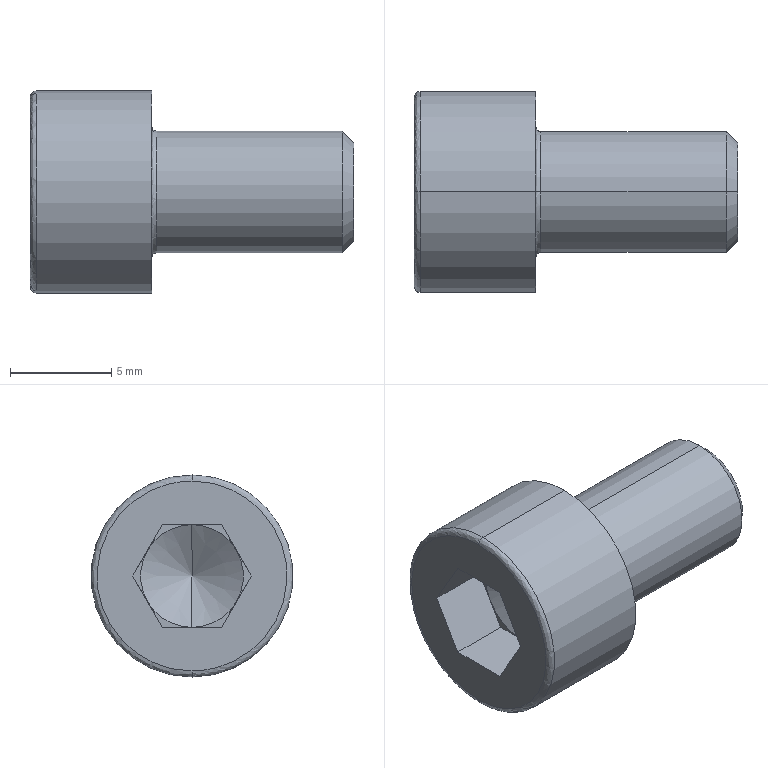Part | SolidWorks | features BaseBody 1 | 1 solid | 27 faces | box 16 x 10 x 10 mm | volume 673.863 mm3 | plane 15 | spline 4 | cylinder 4 | cone 4 | commonest cylinder face diameters 6 x2 10 x2
STEP:
#1=CARTESIAN_POINT('',(0.,0.,4.7));
#2=VERTEX_POINT('',#1);
#3=CARTESIAN_POINT('',(0.,0.,-4.7));
#4=VERTEX_POINT('',#3);
#5=CARTESIAN_POINT('',(0.,0.,4.7));
#6=CARTESIAN_POINT('',(0.,-9.4,4.7));
#7=CARTESIAN_POINT('',(0.,-9.4,-4.7));
#8=CARTESIAN_POINT('',(0.,0.,-4.7));
#9=(BOUNDED_CURVE()B_SPLINE_CURVE(3,(#5,#6,#7,#8),.UNSPECIFIED.,.F.,.F.)B_SPLINE_CURVE_WITH_KNOTS((4,4),(0.,1.),.UNSPECIFIED.)CURVE()GEOMETRIC_REPRESENTATION_ITEM()RATIONAL_B_SPLINE_CURVE((1.,0.3333,0.3333,1.))REPRESENTATION_ITEM(''));
#10=EDGE_CURVE('',#2,#4,#9,.T.);
#11=ORIENTED_EDGE('',*,*,#10,.T.);
#12=CARTESIAN_POINT('',(0.3,0.,-5.));
#13=VERTEX_POINT('',#12);
#14=CARTESIAN_POINT('',(0.3,0.,-4.7));
#15=DIRECTION('',(0.,-1.,0.));
#16=DIRECTION('',(0.,0.,-1.));
#17=AXIS2_PLACEMENT_3D('',#14,#15,#16);
#18=CIRCLE('',#17,0.3);
#19=EDGE_CURVE('',#4,#13,#18,.T.);
#20=ORIENTED_EDGE('',*,*,#19,.T.);
#21=CARTESIAN_POINT('',(0.3,0.,5.));
#22=VERTEX_POINT('',#21);
#23=CARTESIAN_POINT('',(0.3,0.,0.));
#24=DIRECTION('',(1.,0.,0.));
#25=DIRECTION('',(0.,0.,1.));
#26=AXIS2_PLACEMENT_3D('',#23,#24,#25);
#27=CIRCLE('',#26,5.);
#28=EDGE_CURVE('',#22,#13,#27,.T.);
#29=ORIENTED_EDGE('',*,*,#28,.F.);
#30=CARTESIAN_POINT('',(0.3,0.,4.7));
#31=DIRECTION('',(0.,1.,0.));
#32=DIRECTION('',(0.,0.,1.));
#33=AXIS2_PLACEMENT_3D('',#30,#31,#32);
#34=CIRCLE('',#33,0.3);
#35=EDGE_CURVE('',#2,#22,#34,.T.);
#36=ORIENTED_EDGE('',*,*,#35,.F.);
#37=EDGE_LOOP('',(#11,#20,#29,#36));
#38=FACE_OUTER_BOUND('',#37,.T.);
#39=CARTESIAN_POINT('',(0.,0.,-4.7));
#40=CARTESIAN_POINT('',(0.,-9.4,-4.7));
#41=CARTESIAN_POINT('',(0.,-9.4,4.7));
#42=CARTESIAN_POINT('',(0.,0.,4.7));
#43=CARTESIAN_POINT('',(0.,0.,-4.876));
#44=CARTESIAN_POINT('',(0.,-9.751,-4.876));
#45=CARTESIAN_POINT('',(0.,-9.751,4.876));
#46=CARTESIAN_POINT('',(0.,0.,4.876));
#47=CARTESIAN_POINT('',(0.1243,0.,-5.));
#48=CARTESIAN_POINT('',(0.1243,-10.,-5.));
#49=CARTESIAN_POINT('',(0.1243,-10.,5.));
#50=CARTESIAN_POINT('',(0.1243,0.,5.));
#51=CARTESIAN_POINT('',(0.3,0.,-5.));
#52=CARTESIAN_POINT('',(0.3,-10.,-5.));
#53=CARTESIAN_POINT('',(0.3,-10.,5.));
#54=CARTESIAN_POINT('',(0.3,0.,5.));
#55=(BOUNDED_SURFACE()B_SPLINE_SURFACE(3,3,((#39,#40,#41,#42),(#43,#44,#45,#46),(#47,#48,#49,#50),(#51,#52,#53,#54)),.UNSPECIFIED.,.F.,.F.,.T.)B_SPLINE_SURFACE_WITH_KNOTS((4,4),(4,4),(0.,1.),(0.,1.),.UNSPECIFIED.)GEOMETRIC_REPRESENTATION_ITEM()RATIONAL_B_SPLINE_SURFACE(((1.,0.3333,0.3333,1.),(0.8047,0.2682,0.2682,0.8047),(0.8047,0.2682,0.2682,0.8047),(1.,0.3333,0.3333,1.)))REPRESENTATION_ITEM('')SURFACE());
#56=ADVANCED_FACE('',(#38),#55,.T.);
#57=CARTESIAN_POINT('',(6.,0.,3.25));
#58=VERTEX_POINT('',#57);
#59=CARTESIAN_POINT('',(6.,0.,-3.25));
#60=VERTEX_POINT('',#59);
#61=CARTESIAN_POINT('',(6.,0.,3.25));
#62=CARTESIAN_POINT('',(6.,0.2065,3.25));
#63=CARTESIAN_POINT('',(6.,0.511,3.221));
#64=CARTESIAN_POINT('',(6.,0.8568,3.138));
#65=CARTESIAN_POINT('',(6.,1.027,3.084));
#66=CARTESIAN_POINT('',(6.,1.1,3.058));
#67=CARTESIAN_POINT('',(6.,1.148,3.041));
#68=CARTESIAN_POINT('',(6.,1.17,3.032));
#69=CARTESIAN_POINT('',(6.,1.613,2.857));
#70=CARTESIAN_POINT('',(6.,1.981,2.615));
#71=CARTESIAN_POINT('',(6.,2.457,2.14));
#72=CARTESIAN_POINT('',(6.,2.666,1.883));
#73=CARTESIAN_POINT('',(6.,2.861,1.551));
#74=CARTESIAN_POINT('',(6.,2.945,1.376));
#75=CARTESIAN_POINT('',(6.,2.985,1.287));
#76=CARTESIAN_POINT('',(6.,3.001,1.248));
#77=CARTESIAN_POINT('',(6.,3.011,1.222));
#78=CARTESIAN_POINT('',(6.,3.017,1.208));
#79=CARTESIAN_POINT('',(6.,3.174,0.8124));
#80=CARTESIAN_POINT('',(6.,3.25,0.4129));
#81=CARTESIAN_POINT('',(6.,3.25,-0.2065));
#82=CARTESIAN_POINT('',(6.,3.222,-0.5109));
#83=CARTESIAN_POINT('',(6.,3.138,-0.8567));
#84=CARTESIAN_POINT('',(6.,3.084,-1.027));
#85=CARTESIAN_POINT('',(6.,3.058,-1.1));
#86=CARTESIAN_POINT('',(6.,3.041,-1.148));
#87=CARTESIAN_POINT('',(6.,3.032,-1.17));
#88=CARTESIAN_POINT('',(6.,2.857,-1.613));
#89=CARTESIAN_POINT('',(6.,2.615,-1.981));
#90=CARTESIAN_POINT('',(6.,2.14,-2.457));
#91=CARTESIAN_POINT('',(6.,1.883,-2.666));
#92=CARTESIAN_POINT('',(6.,1.551,-2.861));
#93=CARTESIAN_POINT('',(6.,1.376,-2.945));
#94=CARTESIAN_POINT('',(6.,1.3,-2.979));
#95=CARTESIAN_POINT('',(6.,1.248,-3.001));
#96=CARTESIAN_POINT('',(6.,1.22,-3.012));
#97=CARTESIAN_POINT('',(6.,0.8122,-3.174));
#98=CARTESIAN_POINT('',(6.,0.4135,-3.25));
#99=CARTESIAN_POINT('',(6.,0.,-3.25));
#100=B_SPLINE_CURVE_WITH_KNOTS('',3,(#61,#62,#63,#64,#65,#66,#67,#68,#69,#70,#71,#72,#73,#74,#75,#76,#77,#78,#79,#80,#81,#82,#83,#84,#85,#86,#87,#88,#89,#90,#91,#92,#93,#94,#95,#96,#97,#98,#99),.UNSPECIFIED.,.F.,.F.,(4,1,1,1,2,2,2,1,1,1,1,2,2,2,1,1,1,2,2,2,1,1,1,2,2,4),(0.,0.0625,0.09375,0.1094,0.1172,0.125,0.25,0.3125,0.3437,0.3594,0.3672,0.3711,0.375,0.5,0.5625,0.5937,0.6094,0.6172,0.625,0.75,0.8125,0.8438,0.8594,0.8672,0.875,1.),.UNSPECIFIED.);
#101=EDGE_CURVE('',#58,#60,#100,.T.);
#102=ORIENTED_EDGE('',*,*,#101,.F.);
#103=CARTESIAN_POINT('',(6.25,0.,3.));
#104=VERTEX_POINT('',#103);
#105=CARTESIAN_POINT('',(6.25,0.,3.25));
#106=DIRECTION('',(0.,-1.,0.));
#107=DIRECTION('',(0.,0.,1.));
#108=AXIS2_PLACEMENT_3D('',#105,#106,#107);
#109=CIRCLE('',#108,0.25);
#110=EDGE_CURVE('',#58,#104,#109,.T.);
#111=ORIENTED_EDGE('',*,*,#110,.T.);
#112=CARTESIAN_POINT('',(6.25,0.,-3.));
#113=VERTEX_POINT('',#112);
#114=CARTESIAN_POINT('',(6.25,0.,0.));
#115=DIRECTION('',(1.,0.,0.));
#116=DIRECTION('',(0.,0.,-1.));
#117=AXIS2_PLACEMENT_3D('',#114,#115,#116);
#118=CIRCLE('',#117,3.);
#119=EDGE_CURVE('',#113,#104,#118,.T.);
#120=ORIENTED_EDGE('',*,*,#119,.F.);
#121=CARTESIAN_POINT('',(6.25,0.,-3.25));
#122=DIRECTION('',(0.,1.,0.));
#123=DIRECTION('',(0.,0.,-1.));
#124=AXIS2_PLACEMENT_3D('',#121,#122,#123);
#125=CIRCLE('',#124,0.25);
#126=EDGE_CURVE('',#60,#113,#125,.T.);
#127=ORIENTED_EDGE('',*,*,#126,.F.);
#128=EDGE_LOOP('',(#102,#111,#120,#127));
#129=FACE_OUTER_BOUND('',#128,.T.);
#130=CARTESIAN_POINT('',(6.,0.,-3.25));
#131=CARTESIAN_POINT('',(6.,6.5,-3.25));
#132=CARTESIAN_POINT('',(6.,6.5,3.25));
#133=CARTESIAN_POINT('',(6.,0.,3.25));
#134=CARTESIAN_POINT('',(6.,0.,-3.104));
#135=CARTESIAN_POINT('',(6.,6.207,-3.104));
#136=CARTESIAN_POINT('',(6.,6.207,3.104));
#137=CARTESIAN_POINT('',(6.,0.,3.104));
#138=CARTESIAN_POINT('',(6.104,0.,-3.));
#139=CARTESIAN_POINT('',(6.104,6.,-3.));
#140=CARTESIAN_POINT('',(6.104,6.,3.));
#141=CARTESIAN_POINT('',(6.104,0.,3.));
#142=CARTESIAN_POINT('',(6.25,0.,-3.));
#143=CARTESIAN_POINT('',(6.25,6.,-3.));
#144=CARTESIAN_POINT('',(6.25,6.,3.));
#145=CARTESIAN_POINT('',(6.25,0.,3.));
#146=(BOUNDED_SURFACE()B_SPLINE_SURFACE(3,3,((#130,#131,#132,#133),(#134,#135,#136,#137),(#138,#139,#140,#141),(#142,#143,#144,#145)),.UNSPECIFIED.,.F.,.F.,.F.)B_SPLINE_SURFACE_WITH_KNOTS((4,4),(4,4),(0.,1.),(0.,1.),.UNSPECIFIED.)GEOMETRIC_REPRESENTATION_ITEM()RATIONAL_B_SPLINE_SURFACE(((1.,0.3333,0.3333,1.),(0.8047,0.2682,0.2682,0.8047),(0.8047,0.2682,0.2682,0.8047),(1.,0.3333,0.3333,1.)))REPRESENTATION_ITEM('')SURFACE());
#147=ADVANCED_FACE('',(#129),#146,.F.);
#148=CARTESIAN_POINT('',(6.,0.,5.));
#149=VERTEX_POINT('',#148);
#150=CARTESIAN_POINT('',(6.,0.,-5.));
#151=VERTEX_POINT('',#150);
#152=CARTESIAN_POINT('',(6.,0.,0.));
#153=DIRECTION('',(-1.,0.,0.));
#154=DIRECTION('',(0.,0.,1.));
#155=AXIS2_PLACEMENT_3D('',#152,#153,#154);
#156=CIRCLE('',#155,5.);
#157=EDGE_CURVE('',#149,#151,#156,.T.);
#158=ORIENTED_EDGE('',*,*,#157,.T.);
#159=CARTESIAN_POINT('',(-31.75,0.,-5.));
#160=DIRECTION('',(-1.,0.,0.));
#161=VECTOR('',#160,1000.);
#162=LINE('',#159,#161);
#163=EDGE_CURVE('',#151,#13,#162,.T.);
#164=ORIENTED_EDGE('',*,*,#163,.T.);
#165=CARTESIAN_POINT('',(0.3,0.,0.));
#166=DIRECTION('',(1.,0.,0.));
#167=DIRECTION('',(0.,0.,1.));
#168=AXIS2_PLACEMENT_3D('',#165,#166,#167);
#169=CIRCLE('',#168,5.);
#170=EDGE_CURVE('',#13,#22,#169,.T.);
#171=ORIENTED_EDGE('',*,*,#170,.T.);
#172=CARTESIAN_POINT('',(-31.75,0.,5.));
#173=DIRECTION('',(-1.,0.,0.));
#174=VECTOR('',#173,1000.);
#175=LINE('',#172,#174);
#176=EDGE_CURVE('',#149,#22,#175,.T.);
#177=ORIENTED_EDGE('',*,*,#176,.F.);
#178=EDGE_LOOP('',(#158,#164,#171,#177));
#179=FACE_OUTER_BOUND('',#178,.T.);
#180=CARTESIAN_POINT('',(-31.75,0.,0.));
#181=DIRECTION('',(-1.,0.,0.));
#182=DIRECTION('',(0.,0.,1.));
#183=AXIS2_PLACEMENT_3D('',#180,#181,#182);
#184=CYLINDRICAL_SURFACE('',#183,5.);
#185=ADVANCED_FACE('',(#179),#184,.T.);
#186=CARTESIAN_POINT('',(15.446,0.,3.));
#187=VERTEX_POINT('',#186);
#188=CARTESIAN_POINT('',(15.446,0.,-3.));
#189=VERTEX_POINT('',#188);
#190=CARTESIAN_POINT('',(15.446,0.,0.));
#191=DIRECTION('',(-1.,0.,0.));
#192=DIRECTION('',(0.,0.,1.));
#193=AXIS2_PLACEMENT_3D('',#190,#191,#192);
#194=CIRCLE('',#193,3.);
#195=EDGE_CURVE('',#187,#189,#194,.T.);
#196=ORIENTED_EDGE('',*,*,#195,.T.);
#197=CARTESIAN_POINT('',(-31.75,0.,-3.));
#198=DIRECTION('',(-1.,0.,0.));
#199=VECTOR('',#198,1000.);
#200=LINE('',#197,#199);
#201=EDGE_CURVE('',#189,#113,#200,.T.);
#202=ORIENTED_EDGE('',*,*,#201,.T.);
#203=ORIENTED_EDGE('',*,*,#119,.T.);
#204=CARTESIAN_POINT('',(-31.75,0.,3.));
#205=DIRECTION('',(-1.,0.,0.));
#206=VECTOR('',#205,1000.);
#207=LINE('',#204,#206);
#208=EDGE_CURVE('',#187,#104,#207,.T.);
#209=ORIENTED_EDGE('',*,*,#208,.F.);
#210=EDGE_LOOP('',(#196,#202,#203,#209));
#211=FACE_OUTER_BOUND('',#210,.T.);
#212=CARTESIAN_POINT('',(-31.75,0.,0.));
#213=DIRECTION('',(-1.,0.,0.));
#214=DIRECTION('',(0.,0.,1.));
#215=AXIS2_PLACEMENT_3D('',#212,#213,#214);
#216=CYLINDRICAL_SURFACE('',#215,3.);
#217=ADVANCED_FACE('',(#211),#216,.T.);
#218=CARTESIAN_POINT('',(16.,0.,2.445));
#219=VERTEX_POINT('',#218);
#220=CARTESIAN_POINT('',(16.,0.,-2.445));
#221=VERTEX_POINT('',#220);
#222=CARTESIAN_POINT('',(16.,0.,0.));
#223=DIRECTION('',(-1.,0.,0.));
#224=DIRECTION('',(0.,0.,1.));
#225=AXIS2_PLACEMENT_3D('',#222,#223,#224);
#226=CIRCLE('',#225,2.445);
#227=EDGE_CURVE('',#219,#221,#226,.T.);
#228=ORIENTED_EDGE('',*,*,#227,.T.);
#229=CARTESIAN_POINT('',(15.446,0.,-3.));
#230=DIRECTION('',(-0.7071,0.,-0.7071));
#231=VECTOR('',#230,1000.);
#232=LINE('',#229,#231);
#233=EDGE_CURVE('',#221,#189,#232,.T.);
#234=ORIENTED_EDGE('',*,*,#233,.T.);
#235=ORIENTED_EDGE('',*,*,#195,.F.);
#236=CARTESIAN_POINT('',(15.446,0.,3.));
#237=DIRECTION('',(-0.7071,0.,0.7071));
#238=VECTOR('',#237,1000.);
#239=LINE('',#236,#238);
#240=EDGE_CURVE('',#219,#187,#239,.T.);
#241=ORIENTED_EDGE('',*,*,#240,.F.);
#242=EDGE_LOOP('',(#228,#234,#235,#241));
#243=FACE_OUTER_BOUND('',#242,.T.);
#244=CARTESIAN_POINT('',(15.446,0.,0.));
#245=DIRECTION('',(-1.,0.,0.));
#246=DIRECTION('',(0.,0.,1.));
#247=AXIS2_PLACEMENT_3D('',#244,#245,#246);
#248=CONICAL_SURFACE('',#247,3.,0.7854);
#249=ADVANCED_FACE('',(#243),#248,.T.);
#250=CARTESIAN_POINT('',(4.468,0.,0.));
#251=VERTEX_POINT('',#250);
#252=CARTESIAN_POINT('',(3.,0.,2.542));
#253=VERTEX_POINT('',#252);
#254=CARTESIAN_POINT('',(3.,0.,2.542));
#255=DIRECTION('',(-0.5,0.,0.866));
#256=VECTOR('',#255,1000.);
#257=LINE('',#254,#256);
#258=EDGE_CURVE('',#251,#253,#257,.T.);
#259=ORIENTED_EDGE('',*,*,#258,.F.);
#260=CARTESIAN_POINT('',(3.,0.,-2.542));
#261=VERTEX_POINT('',#260);
#262=CARTESIAN_POINT('',(3.,0.,-2.542));
#263=DIRECTION('',(-0.5,0.,-0.866));
#264=VECTOR('',#263,1000.);
#265=LINE('',#262,#264);
#266=EDGE_CURVE('',#251,#261,#265,.T.);
#267=ORIENTED_EDGE('',*,*,#266,.T.);
#268=CARTESIAN_POINT('',(3.,-2.201,-1.271));
#269=VERTEX_POINT('',#268);
#270=CARTESIAN_POINT('',(3.,0.,0.));
#271=DIRECTION('',(1.,0.,0.));
#272=DIRECTION('',(0.,0.,1.));
#273=AXIS2_PLACEMENT_3D('',#270,#271,#272);
#274=CIRCLE('',#273,2.542);
#275=EDGE_CURVE('',#269,#261,#274,.T.);
#276=ORIENTED_EDGE('',*,*,#275,.F.);
#277=CARTESIAN_POINT('',(3.,-2.201,1.271));
#278=VERTEX_POINT('',#277);
#279=CARTESIAN_POINT('',(3.,0.,0.));
#280=DIRECTION('',(1.,0.,0.));
#281=DIRECTION('',(0.,0.,1.));
#282=AXIS2_PLACEMENT_3D('',#279,#280,#281);
#283=CIRCLE('',#282,2.542);
#284=EDGE_CURVE('',#278,#269,#283,.T.);
#285=ORIENTED_EDGE('',*,*,#284,.F.);
#286=CARTESIAN_POINT('',(3.,0.,0.));
#287=DIRECTION('',(1.,0.,0.));
#288=DIRECTION('',(0.,0.,1.));
#289=AXIS2_PLACEMENT_3D('',#286,#287,#288);
#290=CIRCLE('',#289,2.542);
#291=EDGE_CURVE('',#253,#278,#290,.T.);
#292=ORIENTED_EDGE('',*,*,#291,.F.);
#293=EDGE_LOOP('',(#259,#267,#276,#285,#292));
#294=FACE_OUTER_BOUND('',#293,.T.);
#295=CARTESIAN_POINT('',(3.,0.,0.));
#296=DIRECTION('',(-1.,0.,0.));
#297=DIRECTION('',(0.,0.,1.));
#298=AXIS2_PLACEMENT_3D('',#295,#296,#297);
#299=CONICAL_SURFACE('',#298,2.542,1.047);
#300=ADVANCED_FACE('',(#294),#299,.F.);
#301=ORIENTED_EDGE('',*,*,#163,.F.);
#302=CARTESIAN_POINT('',(6.,0.,0.));
#303=DIRECTION('',(-1.,0.,0.));
#304=DIRECTION('',(0.,0.,1.));
#305=AXIS2_PLACEMENT_3D('',#302,#303,#304);
#306=CIRCLE('',#305,5.);
#307=EDGE_CURVE('',#151,#149,#306,.T.);
#308=ORIENTED_EDGE('',*,*,#307,.T.);
#309=ORIENTED_EDGE('',*,*,#176,.T.);
#310=ORIENTED_EDGE('',*,*,#28,.T.);
#311=EDGE_LOOP('',(#301,#308,#309,#310));
#312=FACE_OUTER_BOUND('',#311,.T.);
#313=CARTESIAN_POINT('',(-31.75,0.,0.));
#314=DIRECTION('',(-1.,0.,0.));
#315=DIRECTION('',(0.,0.,1.));
#316=AXIS2_PLACEMENT_3D('',#313,#314,#315);
#317=CYLINDRICAL_SURFACE('',#316,5.);
#318=ADVANCED_FACE('',(#312),#317,.T.);
#319=ORIENTED_EDGE('',*,*,#19,.F.);
#320=CARTESIAN_POINT('',(0.,0.,-4.7));
#321=CARTESIAN_POINT('',(0.,9.4,-4.7));
#322=CARTESIAN_POINT('',(0.,9.4,4.7));
#323=CARTESIAN_POINT('',(0.,0.,4.7));
#324=(BOUNDED_CURVE()B_SPLINE_CURVE(3,(#320,#321,#322,#323),.UNSPECIFIED.,.F.,.F.)B_SPLINE_CURVE_WITH_KNOTS((4,4),(0.,1.),.UNSPECIFIED.)CURVE()GEOMETRIC_REPRESENTATION_ITEM()RATIONAL_B_SPLINE_CURVE((1.,0.3333,0.3333,1.))REPRESENTATION_ITEM(''));
#325=EDGE_CURVE('',#4,#2,#324,.T.);
#326=ORIENTED_EDGE('',*,*,#325,.T.);
#327=ORIENTED_EDGE('',*,*,#35,.T.);
#328=ORIENTED_EDGE('',*,*,#170,.F.);
#329=EDGE_LOOP('',(#319,#326,#327,#328));
#330=FACE_OUTER_BOUND('',#329,.T.);
#331=CARTESIAN_POINT('',(0.,0.,4.7));
#332=CARTESIAN_POINT('',(0.,9.4,4.7));
#333=CARTESIAN_POINT('',(0.,9.4,-4.7));
#334=CARTESIAN_POINT('',(0.,0.,-4.7));
#335=CARTESIAN_POINT('',(0.,0.,4.876));
#336=CARTESIAN_POINT('',(0.,9.751,4.876));
#337=CARTESIAN_POINT('',(0.,9.751,-4.876));
#338=CARTESIAN_POINT('',(0.,0.,-4.876));
#339=CARTESIAN_POINT('',(0.1243,0.,5.));
#340=CARTESIAN_POINT('',(0.1243,10.,5.));
#341=CARTESIAN_POINT('',(0.1243,10.,-5.));
#342=CARTESIAN_POINT('',(0.1243,0.,-5.));
#343=CARTESIAN_POINT('',(0.3,0.,5.));
#344=CARTESIAN_POINT('',(0.3,10.,5.));
#345=CARTESIAN_POINT('',(0.3,10.,-5.));
#346=CARTESIAN_POINT('',(0.3,0.,-5.));
#347=(BOUNDED_SURFACE()B_SPLINE_SURFACE(3,3,((#331,#332,#333,#334),(#335,#336,#337,#338),(#339,#340,#341,#342),(#343,#344,#345,#346)),.UNSPECIFIED.,.F.,.F.,.T.)B_SPLINE_SURFACE_WITH_KNOTS((4,4),(4,4),(0.,1.),(0.,1.),.UNSPECIFIED.)GEOMETRIC_REPRESENTATION_ITEM()RATIONAL_B_SPLINE_SURFACE(((1.,0.3333,0.3333,1.),(0.8047,0.2682,0.2682,0.8047),(0.8047,0.2682,0.2682,0.8047),(1.,0.3333,0.3333,1.)))REPRESENTATION_ITEM('')SURFACE());
#348=ADVANCED_FACE('',(#330),#347,.T.);
#349=ORIENTED_EDGE('',*,*,#157,.F.);
#350=ORIENTED_EDGE('',*,*,#307,.F.);
#351=EDGE_LOOP('',(#349,#350));
#352=FACE_OUTER_BOUND('',#351,.T.);
#353=CARTESIAN_POINT('',(6.,0.,-3.25));
#354=CARTESIAN_POINT('',(6.,-0.2065,-3.25));
#355=CARTESIAN_POINT('',(6.,-0.511,-3.221));
#356=CARTESIAN_POINT('',(6.,-0.8568,-3.138));
#357=CARTESIAN_POINT('',(6.,-1.027,-3.084));
#358=CARTESIAN_POINT('',(6.,-1.1,-3.058));
#359=CARTESIAN_POINT('',(6.,-1.148,-3.041));
#360=CARTESIAN_POINT('',(6.,-1.17,-3.032));
#361=CARTESIAN_POINT('',(6.,-1.613,-2.857));
#362=CARTESIAN_POINT('',(6.,-1.981,-2.615));
#363=CARTESIAN_POINT('',(6.,-2.457,-2.14));
#364=CARTESIAN_POINT('',(6.,-2.666,-1.883));
#365=CARTESIAN_POINT('',(6.,-2.861,-1.551));
#366=CARTESIAN_POINT('',(6.,-2.945,-1.376));
#367=CARTESIAN_POINT('',(6.,-2.985,-1.287));
#368=CARTESIAN_POINT('',(6.,-3.001,-1.248));
#369=CARTESIAN_POINT('',(6.,-3.011,-1.222));
#370=CARTESIAN_POINT('',(6.,-3.017,-1.208));
#371=CARTESIAN_POINT('',(6.,-3.174,-0.8124));
#372=CARTESIAN_POINT('',(6.,-3.25,-0.4129));
#373=CARTESIAN_POINT('',(6.,-3.25,0.2065));
#374=CARTESIAN_POINT('',(6.,-3.222,0.5109));
#375=CARTESIAN_POINT('',(6.,-3.138,0.8567));
#376=CARTESIAN_POINT('',(6.,-3.084,1.027));
#377=CARTESIAN_POINT('',(6.,-3.058,1.1));
#378=CARTESIAN_POINT('',(6.,-3.041,1.148));
#379=CARTESIAN_POINT('',(6.,-3.032,1.17));
#380=CARTESIAN_POINT('',(6.,-2.857,1.613));
#381=CARTESIAN_POINT('',(6.,-2.615,1.981));
#382=CARTESIAN_POINT('',(6.,-2.14,2.457));
#383=CARTESIAN_POINT('',(6.,-1.883,2.666));
#384=CARTESIAN_POINT('',(6.,-1.551,2.861));
#385=CARTESIAN_POINT('',(6.,-1.376,2.945));
#386=CARTESIAN_POINT('',(6.,-1.3,2.979));
#387=CARTESIAN_POINT('',(6.,-1.248,3.001));
#388=CARTESIAN_POINT('',(6.,-1.22,3.012));
#389=CARTESIAN_POINT('',(6.,-0.8122,3.174));
#390=CARTESIAN_POINT('',(6.,-0.4135,3.25));
#391=CARTESIAN_POINT('',(6.,0.,3.25));
#392=B_SPLINE_CURVE_WITH_KNOTS('',3,(#353,#354,#355,#356,#357,#358,#359,#360,#361,#362,#363,#364,#365,#366,#367,#368,#369,#370,#371,#372,#373,#374,#375,#376,#377,#378,#379,#380,#381,#382,#383,#384,#385,#386,#387,#388,#389,#390,#391),.UNSPECIFIED.,.F.,.F.,(4,1,1,1,2,2,2,1,1,1,1,2,2,2,1,1,1,2,2,2,1,1,1,2,2,4),(0.,0.0625,0.09375,0.1094,0.1172,0.125,0.25,0.3125,0.3438,0.3594,0.3672,0.3711,0.375,0.5,0.5625,0.5937,0.6094,0.6172,0.625,0.75,0.8125,0.8437,0.8594,0.8672,0.875,1.),.UNSPECIFIED.);
#393=EDGE_CURVE('',#60,#58,#392,.T.);
#394=ORIENTED_EDGE('',*,*,#393,.T.);
#395=ORIENTED_EDGE('',*,*,#101,.T.);
#396=EDGE_LOOP('',(#394,#395));
#397=FACE_BOUND('',#396,.T.);
#398=CARTESIAN_POINT('',(6.,5.,0.));
#399=DIRECTION('',(1.,0.,0.));
#400=DIRECTION('',(0.,0.,-1.));
#401=AXIS2_PLACEMENT_3D('',#398,#399,#400);
#402=PLANE('',#401);
#403=ADVANCED_FACE('',(#352,#397),#402,.T.);
#404=ORIENTED_EDGE('',*,*,#325,.F.);
#405=ORIENTED_EDGE('',*,*,#10,.F.);
#406=EDGE_LOOP('',(#404,#405));
#407=FACE_OUTER_BOUND('',#406,.T.);
#408=CARTESIAN_POINT('',(0.,-1.468,-2.542));
#409=VERTEX_POINT('',#408);
#410=CARTESIAN_POINT('',(0.,1.468,-2.542));
#411=VERTEX_POINT('',#410);
#412=CARTESIAN_POINT('',(0.,0.,-2.542));
#413=DIRECTION('',(0.,1.,0.));
#414=VECTOR('',#413,1000.);
#415=LINE('',#412,#414);
#416=EDGE_CURVE('',#409,#411,#415,.T.);
#417=ORIENTED_EDGE('',*,*,#416,.T.);
#418=CARTESIAN_POINT('',(0.,2.935,0.));
#419=VERTEX_POINT('',#418);
#420=CARTESIAN_POINT('',(0.,1.468,-2.542));
#421=DIRECTION('',(0.,0.5,0.866));
#422=VECTOR('',#421,1000.);
#423=LINE('',#420,#422);
#424=EDGE_CURVE('',#411,#419,#423,.T.);
#425=ORIENTED_EDGE('',*,*,#424,.T.);
#426=CARTESIAN_POINT('',(0.,1.468,2.542));
#427=VERTEX_POINT('',#426);
#428=CARTESIAN_POINT('',(0.,2.935,0.));
#429=DIRECTION('',(0.,-0.5,0.866));
#430=VECTOR('',#429,1000.);
#431=LINE('',#428,#430);
#432=EDGE_CURVE('',#419,#427,#431,.T.);
#433=ORIENTED_EDGE('',*,*,#432,.T.);
#434=CARTESIAN_POINT('',(0.,-1.468,2.542));
#435=VERTEX_POINT('',#434);
#436=CARTESIAN_POINT('',(0.,0.,2.542));
#437=DIRECTION('',(0.,-1.,0.));
#438=VECTOR('',#437,1000.);
#439=LINE('',#436,#438);
#440=EDGE_CURVE('',#427,#435,#439,.T.);
#441=ORIENTED_EDGE('',*,*,#440,.T.);
#442=CARTESIAN_POINT('',(0.,-2.935,0.));
#443=VERTEX_POINT('',#442);
#444=CARTESIAN_POINT('',(0.,-1.468,2.542));
#445=DIRECTION('',(0.,-0.5,-0.866));
#446=VECTOR('',#445,1000.);
#447=LINE('',#444,#446);
#448=EDGE_CURVE('',#435,#443,#447,.T.);
#449=ORIENTED_EDGE('',*,*,#448,.T.);
#450=CARTESIAN_POINT('',(0.,-2.935,0.));
#451=DIRECTION('',(0.,0.5,-0.866));
#452=VECTOR('',#451,1000.);
#453=LINE('',#450,#452);
#454=EDGE_CURVE('',#443,#409,#453,.T.);
#455=ORIENTED_EDGE('',*,*,#454,.T.);
#456=EDGE_LOOP('',(#417,#425,#433,#441,#449,#455));
#457=FACE_BOUND('',#456,.T.);
#458=CARTESIAN_POINT('',(0.,0.,0.));
#459=DIRECTION('',(-1.,0.,0.));
#460=DIRECTION('',(0.,0.,1.));
#461=AXIS2_PLACEMENT_3D('',#458,#459,#460);
#462=PLANE('',#461);
#463=ADVANCED_FACE('',(#407,#457),#462,.T.);
#464=ORIENTED_EDGE('',*,*,#110,.F.);
#465=ORIENTED_EDGE('',*,*,#393,.F.);
#466=ORIENTED_EDGE('',*,*,#126,.T.);
#467=CARTESIAN_POINT('',(6.25,0.,0.));
#468=DIRECTION('',(1.,0.,0.));
#469=DIRECTION('',(0.,0.,-1.));
#470=AXIS2_PLACEMENT_3D('',#467,#468,#469);
#471=CIRCLE('',#470,3.);
#472=EDGE_CURVE('',#104,#113,#471,.T.);
#473=ORIENTED_EDGE('',*,*,#472,.F.);
#474=EDGE_LOOP('',(#464,#465,#466,#473));
#475=FACE_OUTER_BOUND('',#474,.T.);
#476=CARTESIAN_POINT('',(6.,0.,3.25));
#477=CARTESIAN_POINT('',(6.,-6.5,3.25));
#478=CARTESIAN_POINT('',(6.,-6.5,-3.25));
#479=CARTESIAN_POINT('',(6.,0.,-3.25));
#480=CARTESIAN_POINT('',(6.,0.,3.104));
#481=CARTESIAN_POINT('',(6.,-6.207,3.104));
#482=CARTESIAN_POINT('',(6.,-6.207,-3.104));
#483=CARTESIAN_POINT('',(6.,0.,-3.104));
#484=CARTESIAN_POINT('',(6.104,0.,3.));
#485=CARTESIAN_POINT('',(6.104,-6.,3.));
#486=CARTESIAN_POINT('',(6.104,-6.,-3.));
#487=CARTESIAN_POINT('',(6.104,0.,-3.));
#488=CARTESIAN_POINT('',(6.25,0.,3.));
#489=CARTESIAN_POINT('',(6.25,-6.,3.));
#490=CARTESIAN_POINT('',(6.25,-6.,-3.));
#491=CARTESIAN_POINT('',(6.25,0.,-3.));
#492=(BOUNDED_SURFACE()B_SPLINE_SURFACE(3,3,((#476,#477,#478,#479),(#480,#481,#482,#483),(#484,#485,#486,#487),(#488,#489,#490,#491)),.UNSPECIFIED.,.F.,.F.,.F.)B_SPLINE_SURFACE_WITH_KNOTS((4,4),(4,4),(0.,1.),(0.,1.),.UNSPECIFIED.)GEOMETRIC_REPRESENTATION_ITEM()RATIONAL_B_SPLINE_SURFACE(((1.,0.3333,0.3333,1.),(0.8047,0.2682,0.2682,0.8047),(0.8047,0.2682,0.2682,0.8047),(1.,0.3333,0.3333,1.)))REPRESENTATION_ITEM('')SURFACE());
#493=ADVANCED_FACE('',(#475),#492,.F.);
#494=CARTESIAN_POINT('',(3.,1.468,-2.542));
#495=VERTEX_POINT('',#494);
#496=CARTESIAN_POINT('',(3.,1.468,-2.542));
#497=DIRECTION('',(-1.,0.,0.));
#498=VECTOR('',#497,1000.);
#499=LINE('',#496,#498);
#500=EDGE_CURVE('',#495,#411,#499,.T.);
#501=ORIENTED_EDGE('',*,*,#500,.F.);
#502=CARTESIAN_POINT('',(3.,2.201,-1.271));
#503=VERTEX_POINT('',#502);
#504=CARTESIAN_POINT('',(3.,1.468,-2.542));
#505=DIRECTION('',(0.,0.5,0.866));
#506=VECTOR('',#505,1000.);
#507=LINE('',#504,#506);
#508=EDGE_CURVE('',#495,#503,#507,.T.);
#509=ORIENTED_EDGE('',*,*,#508,.T.);
#510=CARTESIAN_POINT('',(3.,2.935,0.));
#511=VERTEX_POINT('',#510);
#512=CARTESIAN_POINT('',(3.,2.201,-1.271));
#513=DIRECTION('',(0.,0.5,0.866));
#514=VECTOR('',#513,1000.);
#515=LINE('',#512,#514);
#516=EDGE_CURVE('',#503,#511,#515,.T.);
#517=ORIENTED_EDGE('',*,*,#516,.T.);
#518=CARTESIAN_POINT('',(3.,2.935,0.));
#519=DIRECTION('',(1.,0.,0.));
#520=VECTOR('',#519,1000.);
#521=LINE('',#518,#520);
#522=EDGE_CURVE('',#419,#511,#521,.T.);
#523=ORIENTED_EDGE('',*,*,#522,.F.);
#524=ORIENTED_EDGE('',*,*,#424,.F.);
#525=EDGE_LOOP('',(#501,#509,#517,#523,#524));
#526=FACE_OUTER_BOUND('',#525,.T.);
#527=CARTESIAN_POINT('',(3.,2.935,0.));
#528=DIRECTION('',(0.,0.866,-0.5));
#529=DIRECTION('',(0.,0.5,0.866));
#530=AXIS2_PLACEMENT_3D('',#527,#528,#529);
#531=PLANE('',#530);
#532=ADVANCED_FACE('',(#526),#531,.F.);
#533=CARTESIAN_POINT('',(3.,-1.468,-2.542));
#534=VERTEX_POINT('',#533);
#535=CARTESIAN_POINT('',(3.,-1.468,-2.542));
#536=DIRECTION('',(-1.,0.,0.));
#537=VECTOR('',#536,1000.);
#538=LINE('',#535,#537);
#539=EDGE_CURVE('',#534,#409,#538,.T.);
#540=ORIENTED_EDGE('',*,*,#539,.F.);
#541=CARTESIAN_POINT('',(3.,2.935,-2.542));
#542=DIRECTION('',(0.,1.,0.));
#543=VECTOR('',#542,1000.);
#544=LINE('',#541,#543);
#545=EDGE_CURVE('',#534,#261,#544,.T.);
#546=ORIENTED_EDGE('',*,*,#545,.T.);
#547=CARTESIAN_POINT('',(3.,2.935,-2.542));
#548=DIRECTION('',(0.,1.,0.));
#549=VECTOR('',#548,1000.);
#550=LINE('',#547,#549);
#551=EDGE_CURVE('',#261,#495,#550,.T.);
#552=ORIENTED_EDGE('',*,*,#551,.T.);
#553=ORIENTED_EDGE('',*,*,#500,.T.);
#554=ORIENTED_EDGE('',*,*,#416,.F.);
#555=EDGE_LOOP('',(#540,#546,#552,#553,#554));
#556=FACE_OUTER_BOUND('',#555,.T.);
#557=CARTESIAN_POINT('',(3.,1.468,-2.542));
#558=DIRECTION('',(0.,0.,-1.));
#559=DIRECTION('',(0.,1.,0.));
#560=AXIS2_PLACEMENT_3D('',#557,#558,#559);
#561=PLANE('',#560);
#562=ADVANCED_FACE('',(#556),#561,.F.);
#563=CARTESIAN_POINT('',(3.,-2.201,-1.271));
#564=DIRECTION('',(0.,0.5,-0.866));
#565=VECTOR('',#564,1000.);
#566=LINE('',#563,#565);
#567=EDGE_CURVE('',#269,#534,#566,.T.);
#568=ORIENTED_EDGE('',*,*,#567,.T.);
#569=ORIENTED_EDGE('',*,*,#539,.T.);
#570=ORIENTED_EDGE('',*,*,#454,.F.);
#571=CARTESIAN_POINT('',(3.,-2.935,0.));
#572=VERTEX_POINT('',#571);
#573=CARTESIAN_POINT('',(3.,-2.935,0.));
#574=DIRECTION('',(1.,0.,0.));
#575=VECTOR('',#574,1000.);
#576=LINE('',#573,#575);
#577=EDGE_CURVE('',#443,#572,#576,.T.);
#578=ORIENTED_EDGE('',*,*,#577,.T.);
#579=CARTESIAN_POINT('',(3.,-2.935,0.));
#580=DIRECTION('',(0.,0.5,-0.866));
#581=VECTOR('',#580,1000.);
#582=LINE('',#579,#581);
#583=EDGE_CURVE('',#572,#269,#582,.T.);
#584=ORIENTED_EDGE('',*,*,#583,.T.);
#585=EDGE_LOOP('',(#568,#569,#570,#578,#584));
#586=FACE_OUTER_BOUND('',#585,.T.);
#587=CARTESIAN_POINT('',(3.,-2.935,0.));
#588=DIRECTION('',(0.,0.866,0.5));
#589=DIRECTION('',(0.,-0.5,0.866));
#590=AXIS2_PLACEMENT_3D('',#587,#588,#589);
#591=PLANE('',#590);
#592=ADVANCED_FACE('',(#586),#591,.T.);
#593=CARTESIAN_POINT('',(3.,-2.201,1.271));
#594=DIRECTION('',(0.,-0.5,-0.866));
#595=VECTOR('',#594,1000.);
#596=LINE('',#593,#595);
#597=EDGE_CURVE('',#278,#572,#596,.T.);
#598=ORIENTED_EDGE('',*,*,#597,.T.);
#599=ORIENTED_EDGE('',*,*,#577,.F.);
#600=ORIENTED_EDGE('',*,*,#448,.F.);
#601=CARTESIAN_POINT('',(3.,-1.468,2.542));
#602=VERTEX_POINT('',#601);
#603=CARTESIAN_POINT('',(3.,-1.468,2.542));
#604=DIRECTION('',(1.,0.,0.));
#605=VECTOR('',#604,1000.);
#606=LINE('',#603,#605);
#607=EDGE_CURVE('',#435,#602,#606,.T.);
#608=ORIENTED_EDGE('',*,*,#607,.T.);
#609=CARTESIAN_POINT('',(3.,-1.468,2.542));
#610=DIRECTION('',(0.,-0.5,-0.866));
#611=VECTOR('',#610,1000.);
#612=LINE('',#609,#611);
#613=EDGE_CURVE('',#602,#278,#612,.T.);
#614=ORIENTED_EDGE('',*,*,#613,.T.);
#615=EDGE_LOOP('',(#598,#599,#600,#608,#614));
#616=FACE_OUTER_BOUND('',#615,.T.);
#617=CARTESIAN_POINT('',(3.,-1.468,2.542));
#618=DIRECTION('',(0.,0.866,-0.5));
#619=DIRECTION('',(0.,0.5,0.866));
#620=AXIS2_PLACEMENT_3D('',#617,#618,#619);
#621=PLANE('',#620);
#622=ADVANCED_FACE('',(#616),#621,.T.);
#623=CARTESIAN_POINT('',(3.,1.468,2.542));
#624=VERTEX_POINT('',#623);
#625=CARTESIAN_POINT('',(3.,1.468,2.542));
#626=DIRECTION('',(-1.,0.,0.));
#627=VECTOR('',#626,1000.);
#628=LINE('',#625,#627);
#629=EDGE_CURVE('',#624,#427,#628,.T.);
#630=ORIENTED_EDGE('',*,*,#629,.F.);
#631=CARTESIAN_POINT('',(3.,-1.468,2.542));
#632=DIRECTION('',(0.,1.,0.));
#633=VECTOR('',#632,1000.);
#634=LINE('',#631,#633);
#635=EDGE_CURVE('',#253,#624,#634,.T.);
#636=ORIENTED_EDGE('',*,*,#635,.F.);
#637=CARTESIAN_POINT('',(3.,2.935,2.542));
#638=DIRECTION('',(0.,-1.,0.));
#639=VECTOR('',#638,1000.);
#640=LINE('',#637,#639);
#641=EDGE_CURVE('',#253,#602,#640,.T.);
#642=ORIENTED_EDGE('',*,*,#641,.T.);
#643=ORIENTED_EDGE('',*,*,#607,.F.);
#644=ORIENTED_EDGE('',*,*,#440,.F.);
#645=EDGE_LOOP('',(#630,#636,#642,#643,#644));
#646=FACE_OUTER_BOUND('',#645,.T.);
#647=CARTESIAN_POINT('',(3.,-1.468,2.542));
#648=DIRECTION('',(0.,0.,1.));
#649=DIRECTION('',(0.,-1.,0.));
#650=AXIS2_PLACEMENT_3D('',#647,#648,#649);
#651=PLANE('',#650);
#652=ADVANCED_FACE('',(#646),#651,.F.);
#653=CARTESIAN_POINT('',(3.,2.201,1.271));
#654=VERTEX_POINT('',#653);
#655=CARTESIAN_POINT('',(3.,2.935,0.));
#656=DIRECTION('',(0.,-0.5,0.866));
#657=VECTOR('',#656,1000.);
#658=LINE('',#655,#657);
#659=EDGE_CURVE('',#654,#624,#658,.T.);
#660=ORIENTED_EDGE('',*,*,#659,.T.);
#661=ORIENTED_EDGE('',*,*,#629,.T.);
#662=ORIENTED_EDGE('',*,*,#432,.F.);
#663=ORIENTED_EDGE('',*,*,#522,.T.);
#664=CARTESIAN_POINT('',(3.,2.935,0.));
#665=DIRECTION('',(0.,-0.5,0.866));
#666=VECTOR('',#665,1000.);
#667=LINE('',#664,#666);
#668=EDGE_CURVE('',#511,#654,#667,.T.);
#669=ORIENTED_EDGE('',*,*,#668,.T.);
#670=EDGE_LOOP('',(#660,#661,#662,#663,#669));
#671=FACE_OUTER_BOUND('',#670,.T.);
#672=CARTESIAN_POINT('',(3.,2.935,0.));
#673=DIRECTION('',(0.,-0.866,-0.5));
#674=DIRECTION('',(0.,0.5,-0.866));
#675=AXIS2_PLACEMENT_3D('',#672,#673,#674);
#676=PLANE('',#675);
#677=ADVANCED_FACE('',(#671),#676,.T.);
#678=ORIENTED_EDGE('',*,*,#201,.F.);
#679=CARTESIAN_POINT('',(15.446,0.,0.));
#680=DIRECTION('',(-1.,0.,0.));
#681=DIRECTION('',(0.,0.,1.));
#682=AXIS2_PLACEMENT_3D('',#679,#680,#681);
#683=CIRCLE('',#682,3.);
#684=EDGE_CURVE('',#189,#187,#683,.T.);
#685=ORIENTED_EDGE('',*,*,#684,.T.);
#686=ORIENTED_EDGE('',*,*,#208,.T.);
#687=ORIENTED_EDGE('',*,*,#472,.T.);
#688=EDGE_LOOP('',(#678,#685,#686,#687));
#689=FACE_OUTER_BOUND('',#688,.T.);
#690=CARTESIAN_POINT('',(-31.75,0.,0.));
#691=DIRECTION('',(-1.,0.,0.));
#692=DIRECTION('',(0.,0.,1.));
#693=AXIS2_PLACEMENT_3D('',#690,#691,#692);
#694=CYLINDRICAL_SURFACE('',#693,3.);
#695=ADVANCED_FACE('',(#689),#694,.T.);
#696=ORIENTED_EDGE('',*,*,#659,.F.);
#697=CARTESIAN_POINT('',(3.,0.,0.));
#698=DIRECTION('',(-1.,0.,0.));
#699=DIRECTION('',(0.,0.,1.));
#700=AXIS2_PLACEMENT_3D('',#697,#698,#699);
#701=CIRCLE('',#700,2.542);
#702=EDGE_CURVE('',#253,#654,#701,.T.);
#703=ORIENTED_EDGE('',*,*,#702,.F.);
#704=ORIENTED_EDGE('',*,*,#635,.T.);
#705=EDGE_LOOP('',(#696,#703,#704));
#706=FACE_OUTER_BOUND('',#705,.T.);
#707=CARTESIAN_POINT('',(3.,2.935,0.));
#708=DIRECTION('',(1.,0.,0.));
#709=DIRECTION('',(0.,0.,-1.));
#710=AXIS2_PLACEMENT_3D('',#707,#708,#709);
#711=PLANE('',#710);
#712=ADVANCED_FACE('',(#706),#711,.F.);
#713=ORIENTED_EDGE('',*,*,#233,.F.);
#714=CARTESIAN_POINT('',(16.,0.,0.));
#715=DIRECTION('',(-1.,0.,0.));
#716=DIRECTION('',(0.,0.,1.));
#717=AXIS2_PLACEMENT_3D('',#714,#715,#716);
#718=CIRCLE('',#717,2.445);
#719=EDGE_CURVE('',#221,#219,#718,.T.);
#720=ORIENTED_EDGE('',*,*,#719,.T.);
#721=ORIENTED_EDGE('',*,*,#240,.T.);
#722=ORIENTED_EDGE('',*,*,#684,.F.);
#723=EDGE_LOOP('',(#713,#720,#721,#722));
#724=FACE_OUTER_BOUND('',#723,.T.);
#725=CARTESIAN_POINT('',(15.446,0.,0.));
#726=DIRECTION('',(-1.,0.,0.));
#727=DIRECTION('',(0.,0.,1.));
#728=AXIS2_PLACEMENT_3D('',#725,#726,#727);
#729=CONICAL_SURFACE('',#728,3.,0.7854);
#730=ADVANCED_FACE('',(#724),#729,.T.);
#731=ORIENTED_EDGE('',*,*,#266,.F.);
#732=ORIENTED_EDGE('',*,*,#258,.T.);
#733=ORIENTED_EDGE('',*,*,#702,.T.);
#734=CARTESIAN_POINT('',(3.,0.,0.));
#735=DIRECTION('',(1.,0.,0.));
#736=DIRECTION('',(0.,0.,1.));
#737=AXIS2_PLACEMENT_3D('',#734,#735,#736);
#738=CIRCLE('',#737,2.542);
#739=EDGE_CURVE('',#503,#654,#738,.T.);
#740=ORIENTED_EDGE('',*,*,#739,.F.);
#741=CARTESIAN_POINT('',(3.,0.,0.));
#742=DIRECTION('',(1.,0.,0.));
#743=DIRECTION('',(0.,0.,1.));
#744=AXIS2_PLACEMENT_3D('',#741,#742,#743);
#745=CIRCLE('',#744,2.542);
#746=EDGE_CURVE('',#261,#503,#745,.T.);
#747=ORIENTED_EDGE('',*,*,#746,.F.);
#748=EDGE_LOOP('',(#731,#732,#733,#740,#747));
#749=FACE_OUTER_BOUND('',#748,.T.);
#750=CARTESIAN_POINT('',(3.,0.,0.));
#751=DIRECTION('',(-1.,0.,0.));
#752=DIRECTION('',(0.,0.,1.));
#753=AXIS2_PLACEMENT_3D('',#750,#751,#752);
#754=CONICAL_SURFACE('',#753,2.542,1.047);
#755=ADVANCED_FACE('',(#749),#754,.F.);
#756=ORIENTED_EDGE('',*,*,#227,.F.);
#757=ORIENTED_EDGE('',*,*,#719,.F.);
#758=EDGE_LOOP('',(#756,#757));
#759=FACE_OUTER_BOUND('',#758,.T.);
#760=CARTESIAN_POINT('',(16.,2.446,0.));
#761=DIRECTION('',(1.,0.,0.));
#762=DIRECTION('',(0.,0.,-1.));
#763=AXIS2_PLACEMENT_3D('',#760,#761,#762);
#764=PLANE('',#763);
#765=ADVANCED_FACE('',(#759),#764,.T.);
#766=ORIENTED_EDGE('',*,*,#516,.F.);
#767=ORIENTED_EDGE('',*,*,#739,.T.);
#768=ORIENTED_EDGE('',*,*,#668,.F.);
#769=EDGE_LOOP('',(#766,#767,#768));
#770=FACE_OUTER_BOUND('',#769,.T.);
#771=CARTESIAN_POINT('',(3.,2.935,0.));
#772=DIRECTION('',(1.,0.,0.));
#773=DIRECTION('',(0.,0.,-1.));
#774=AXIS2_PLACEMENT_3D('',#771,#772,#773);
#775=PLANE('',#774);
#776=ADVANCED_FACE('',(#770),#775,.F.);
#777=ORIENTED_EDGE('',*,*,#551,.F.);
#778=ORIENTED_EDGE('',*,*,#746,.T.);
#779=ORIENTED_EDGE('',*,*,#508,.F.);
#780=EDGE_LOOP('',(#777,#778,#779));
#781=FACE_OUTER_BOUND('',#780,.T.);
#782=CARTESIAN_POINT('',(3.,2.935,0.));
#783=DIRECTION('',(1.,0.,0.));
#784=DIRECTION('',(0.,0.,-1.));
#785=AXIS2_PLACEMENT_3D('',#782,#783,#784);
#786=PLANE('',#785);
#787=ADVANCED_FACE('',(#781),#786,.F.);
#788=ORIENTED_EDGE('',*,*,#567,.F.);
#789=ORIENTED_EDGE('',*,*,#275,.T.);
#790=ORIENTED_EDGE('',*,*,#545,.F.);
#791=EDGE_LOOP('',(#788,#789,#790));
#792=FACE_OUTER_BOUND('',#791,.T.);
#793=CARTESIAN_POINT('',(3.,2.935,0.));
#794=DIRECTION('',(1.,0.,0.));
#795=DIRECTION('',(0.,0.,-1.));
#796=AXIS2_PLACEMENT_3D('',#793,#794,#795);
#797=PLANE('',#796);
#798=ADVANCED_FACE('',(#792),#797,.F.);
#799=ORIENTED_EDGE('',*,*,#597,.F.);
#800=ORIENTED_EDGE('',*,*,#284,.T.);
#801=ORIENTED_EDGE('',*,*,#583,.F.);
#802=EDGE_LOOP('',(#799,#800,#801));
#803=FACE_OUTER_BOUND('',#802,.T.);
#804=CARTESIAN_POINT('',(3.,2.935,0.));
#805=DIRECTION('',(1.,0.,0.));
#806=DIRECTION('',(0.,0.,-1.));
#807=AXIS2_PLACEMENT_3D('',#804,#805,#806);
#808=PLANE('',#807);
#809=ADVANCED_FACE('',(#803),#808,.F.);
#810=ORIENTED_EDGE('',*,*,#641,.F.);
#811=ORIENTED_EDGE('',*,*,#291,.T.);
#812=ORIENTED_EDGE('',*,*,#613,.F.);
#813=EDGE_LOOP('',(#810,#811,#812));
#814=FACE_OUTER_BOUND('',#813,.T.);
#815=CARTESIAN_POINT('',(3.,2.935,0.));
#816=DIRECTION('',(1.,0.,0.));
#817=DIRECTION('',(0.,0.,-1.));
#818=AXIS2_PLACEMENT_3D('',#815,#816,#817);
#819=PLANE('',#818);
#820=ADVANCED_FACE('',(#814),#819,.F.);
#821=CLOSED_SHELL('',(#56,#147,#185,#217,#249,#300,#318,#348,#403,#463,#493,#532,#562,#592,#622,#652,#677,#695,#712,#730,#755,#765,#776,#787,#798,#809,#820));
#822=MANIFOLD_SOLID_BREP('',#821);
#823=CARTESIAN_POINT('',(0.,0.,0.));
#824=DIRECTION('',(0.,0.,1.));
#825=DIRECTION('',(1.,0.,0.));
#826=AXIS2_PLACEMENT_3D('',#823,#824,#825);
#827=(LENGTH_UNIT()NAMED_UNIT(*)SI_UNIT(.MILLI.,.METRE.));
#828=UNCERTAINTY_MEASURE_WITH_UNIT(LENGTH_MEASURE(0.00001),#827,'','');
#829=(NAMED_UNIT(*)PLANE_ANGLE_UNIT()SI_UNIT($,.RADIAN.));
#830=(NAMED_UNIT(*)SI_UNIT($,.STERADIAN.)SOLID_ANGLE_UNIT());
#831=(GEOMETRIC_REPRESENTATION_CONTEXT(3)GLOBAL_UNCERTAINTY_ASSIGNED_CONTEXT((#828))GLOBAL_UNIT_ASSIGNED_CONTEXT((#827,#829,#830))REPRESENTATION_CONTEXT('',''));
#832=ADVANCED_BREP_SHAPE_REPRESENTATION('',(#822,#826),#831);